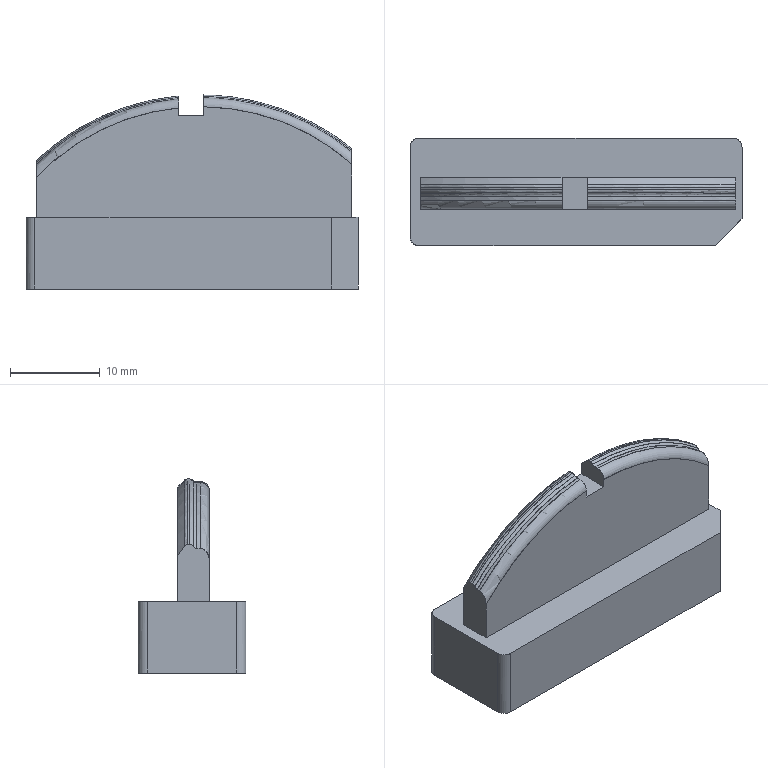CAM job | PowerMill | 3-axis milling, other | part box 37 x 12 x 21.629 mm
Tools:
number,name,type,diameter,tip_radius,length,cutting_length,overhang,flutes,holder,toolpaths_using
1,D10C,end_mill,10.0,0.0,60.0,,30.0,1,D42L35,1
2,D4C,end_mill,4.0,0.0,30.0,,15.0,1,D42L35,1
1,D10C_1_1_1,end_mill,10.0,0.0,60.0,,22.08,1,D42L35,3
2,D4C_1_1,end_mill,4.0,0.0,30.0,,13.8,1,D42L35,1
28,D2C_1_1,end_mill,2.0,0.0,3.0,,2.56,1,D42L35,1
3,D10_1_1_1,end_mill,10.0,0.0,60.0,,21.8,1,D42L35,3
4,R1_1_1,ball_nosed,2.0,1.0,3.0,,10.24,1,D42L35,1
12,D2_1_1,end_mill,2.0,0.0,3.0,,2.68,1,D42L35,1
6,R0.5_1_1,ball_nosed,1.0,0.5,3.0,,8.2,1,D42L35,1
13,Text_D4_1_1,taper_spherical,4.0,0.3,60.0,,13.88,1,D42L35,1
Operations:
program,toolpath,strategy,tool,tool_number,tool_diameter,tip_radius,flutes,spindle_rpm,feed_cut,surface_speed_m_min_computed,feed_per_tooth_computed,tolerance,thickness,stepover,stepdown,cut_length,cut_time_min,total_time_min,workplane
19-0709-5-F,精公开粗01-扫面平行-D10C,raster_area_clear,D10C_1_1_1,1,10.0,0.0,1.0,8000.0,10000.0,251.33,1.25,0.03,0.28,6.0,1.0,187.8,0.019,0.0247,
19-0709-5-F,精公开粗01-外形偏置-D10C,offset_area_clear,D10C_1_1_1,1,10.0,0.0,1.0,8000.0,10000.0,251.33,1.25,0.03,0.28,6.0,1.0,8510.437,0.851,0.9357,
19-0709-5-F,精公开粗01-基准台等高-D10C,constantz,D10C_1_1_1,1,10.0,0.0,1.0,8000.0,10000.0,251.33,1.25,0.03,0.07,5.0,0.4,2789.004,0.279,0.2889,
19-0709-5-F,精公再粗02-外形偏置-D4C,offset_area_clear,D4C_1_1,2,4.0,0.0,1.0,18000.0,6000.0,226.19,0.3333,0.03,0.0,2.0,1.0,5537.395,0.923,0.9554,
19-0709-5-F,精公再粗03-外形偏置-D2C,offset_area_clear,D2C_1_1,28,2.0,0.0,1.0,18000.0,4000.0,113.1,0.2222,0.03,0.0,1.1,1.0,226.144,0.057,0.0934,
19-0709-5-F,精公基准台01-基准面偏置-D10,offset_area_clear,D10_1_1_1,3,10.0,0.0,1.0,8500.0,600.0,267.04,0.0706,0.005,0.38,5.0,1.0,120.379,0.201,0.2192,
19-0709-5-F,精公基准台01-外形侧光-D10,profile_area_clear,D10_1_1_1,3,10.0,0.0,1.0,8500.0,600.0,267.04,0.0706,0.005,-0.07,0.08,1.0,216.963,0.362,0.3831,
19-0709-5-F,精公基准台01-基准台侧光-D10,profile_area_clear,D10_1_1_1,3,10.0,0.0,1.0,8500.0,600.0,267.04,0.0706,0.005,0.0,0.08,1.0,253.233,0.422,0.4867,
19-0709-5-F,精公精光01-平行-R1,raster,R1_1_1,4,2.0,1.0,1.0,18000.0,2000.0,113.1,0.1111,0.005,-0.075,0.03,1.0,7573.729,3.787,3.821,
19-0709-5-F,精公精光02-等高-D2,constantz,D2_1_1,12,2.0,0.0,1.0,18000.0,1500.0,113.1,0.0833,0.005,-0.075,5.0,0.03,667.213,0.445,0.5626,
19-0709-5-F,精公精光03-清角-R0.5,automatic_corner,R0.5_1_1,6,1.0,0.5,1.0,20000.0,1000.0,62.83,0.05,0.005,-0.075,5.0,1.0,925.514,0.925,0.9495,
19-0709-5-F,精公刻字01-刻字-Text_D4,pattern,Text_D4_1_1,13,4.0,0.3,1.0,15000.0,1000.0,188.5,0.0667,0.005,0.0,5.0,1.0,43.892,0.044,0.0763,
,精公开粗01-外形偏置-D10C_Reference,offset_area_clear,D10C,1,10.0,0.0,1.0,8000.0,10000.0,251.33,1.25,0.03,0.28,6.0,1.0,17004.544,1.701,1.868,
,精公再粗02-外形偏置-D4C_Reference,offset_area_clear,D4C,2,4.0,0.0,1.0,18000.0,6000.0,226.19,0.3333,0.03,0.0,2.0,1.0,10878.572,1.813,1.869,